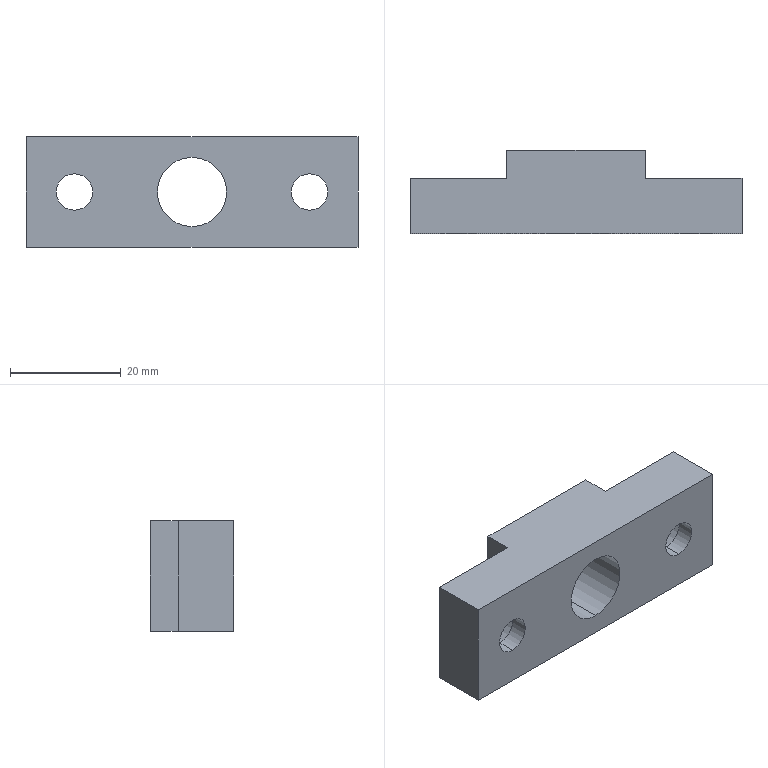Part | STEP file | Knob seat QY-1-21 | 1 solid | 22 faces | box 60 x 15 x 20 mm | volume 11148 mm3 | plane 12 | cylinder 10 | commonest cylinder face diameters 6.6 x4 11 x4 12.5 x2